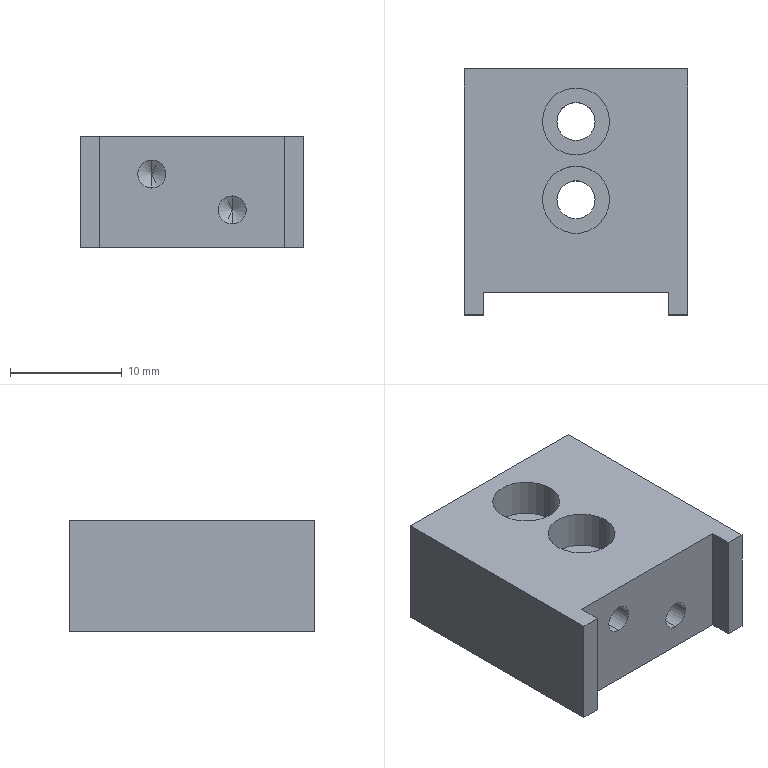Part | SolidWorks | features MBimport 1 | 1 solid | 35 faces | box 20 x 22 x 10 mm | volume 3468 mm3 | plane 16 | cylinder 15 | cone 4 | commonest cylinder face diameters 2.5 x4 3.4 x4 6 x4 3 x3
STEP:
#1=CARTESIAN_POINT('',(3.6,-5.,-0.35));
#2=VERTEX_POINT('',#1);
#3=CARTESIAN_POINT('',(3.6,-5.,-2.85));
#4=VERTEX_POINT('',#3);
#5=CARTESIAN_POINT('',(3.6,-5.,-1.6));
#6=DIRECTION('',(0.,-1.,0.));
#7=DIRECTION('',(0.,0.,-1.));
#8=AXIS2_PLACEMENT_3D('',#5,#6,#7);
#9=CIRCLE('',#8,1.25);
#10=EDGE_CURVE('',#2,#4,#9,.T.);
#11=ORIENTED_EDGE('',*,*,#10,.F.);
#12=CARTESIAN_POINT('',(3.6,-10.,-0.35));
#13=VERTEX_POINT('',#12);
#14=CARTESIAN_POINT('',(3.6,-10.,-0.35));
#15=DIRECTION('',(0.,-1.,0.));
#16=VECTOR('',#15,1000.);
#17=LINE('',#14,#16);
#18=EDGE_CURVE('',#2,#13,#17,.T.);
#19=ORIENTED_EDGE('',*,*,#18,.T.);
#20=CARTESIAN_POINT('',(3.6,-10.,-2.85));
#21=VERTEX_POINT('',#20);
#22=CARTESIAN_POINT('',(3.6,-10.,-1.6));
#23=DIRECTION('',(0.,-1.,0.));
#24=DIRECTION('',(0.,0.,-1.));
#25=AXIS2_PLACEMENT_3D('',#22,#23,#24);
#26=CIRCLE('',#25,1.25);
#27=EDGE_CURVE('',#13,#21,#26,.T.);
#28=ORIENTED_EDGE('',*,*,#27,.T.);
#29=CARTESIAN_POINT('',(3.6,-10.,-2.85));
#30=DIRECTION('',(0.,-1.,0.));
#31=VECTOR('',#30,1000.);
#32=LINE('',#29,#31);
#33=EDGE_CURVE('',#4,#21,#32,.T.);
#34=ORIENTED_EDGE('',*,*,#33,.F.);
#35=EDGE_LOOP('',(#11,#19,#28,#34));
#36=FACE_OUTER_BOUND('',#35,.T.);
#37=CARTESIAN_POINT('',(3.6,-10.,-1.6));
#38=DIRECTION('',(0.,-1.,0.));
#39=DIRECTION('',(0.,0.,-1.));
#40=AXIS2_PLACEMENT_3D('',#37,#38,#39);
#41=CYLINDRICAL_SURFACE('',#40,1.25);
#42=ADVANCED_FACE('',(#36),#41,.F.);
#43=CARTESIAN_POINT('',(3.6,-4.249,-1.6));
#44=VERTEX_POINT('',#43);
#45=CARTESIAN_POINT('',(3.6,-5.,-2.85));
#46=DIRECTION('',(0.,-0.515,-0.8572));
#47=VECTOR('',#46,1000.);
#48=LINE('',#45,#47);
#49=EDGE_CURVE('',#44,#4,#48,.T.);
#50=ORIENTED_EDGE('',*,*,#49,.F.);
#51=CARTESIAN_POINT('',(3.6,-5.,-0.35));
#52=DIRECTION('',(0.,-0.515,0.8572));
#53=VECTOR('',#52,1000.);
#54=LINE('',#51,#53);
#55=EDGE_CURVE('',#44,#2,#54,.T.);
#56=ORIENTED_EDGE('',*,*,#55,.T.);
#57=ORIENTED_EDGE('',*,*,#10,.T.);
#58=EDGE_LOOP('',(#50,#56,#57));
#59=FACE_OUTER_BOUND('',#58,.T.);
#60=CARTESIAN_POINT('',(3.6,-5.,-1.6));
#61=DIRECTION('',(0.,-1.,0.));
#62=DIRECTION('',(0.,0.,-1.));
#63=AXIS2_PLACEMENT_3D('',#60,#61,#62);
#64=CONICAL_SURFACE('',#63,1.25,1.03);
#65=ADVANCED_FACE('',(#59),#64,.F.);
#66=CARTESIAN_POINT('',(-3.6,-5.,2.85));
#67=VERTEX_POINT('',#66);
#68=CARTESIAN_POINT('',(-3.6,-5.,0.35));
#69=VERTEX_POINT('',#68);
#70=CARTESIAN_POINT('',(-3.6,-5.,1.6));
#71=DIRECTION('',(0.,-1.,0.));
#72=DIRECTION('',(0.,0.,-1.));
#73=AXIS2_PLACEMENT_3D('',#70,#71,#72);
#74=CIRCLE('',#73,1.25);
#75=EDGE_CURVE('',#67,#69,#74,.T.);
#76=ORIENTED_EDGE('',*,*,#75,.F.);
#77=CARTESIAN_POINT('',(-3.6,-10.,2.85));
#78=VERTEX_POINT('',#77);
#79=CARTESIAN_POINT('',(-3.6,-10.,2.85));
#80=DIRECTION('',(0.,-1.,0.));
#81=VECTOR('',#80,1000.);
#82=LINE('',#79,#81);
#83=EDGE_CURVE('',#67,#78,#82,.T.);
#84=ORIENTED_EDGE('',*,*,#83,.T.);
#85=CARTESIAN_POINT('',(-3.6,-10.,0.35));
#86=VERTEX_POINT('',#85);
#87=CARTESIAN_POINT('',(-3.6,-10.,1.6));
#88=DIRECTION('',(0.,-1.,0.));
#89=DIRECTION('',(0.,0.,-1.));
#90=AXIS2_PLACEMENT_3D('',#87,#88,#89);
#91=CIRCLE('',#90,1.25);
#92=EDGE_CURVE('',#78,#86,#91,.T.);
#93=ORIENTED_EDGE('',*,*,#92,.T.);
#94=CARTESIAN_POINT('',(-3.6,-10.,0.35));
#95=DIRECTION('',(0.,-1.,0.));
#96=VECTOR('',#95,1000.);
#97=LINE('',#94,#96);
#98=EDGE_CURVE('',#69,#86,#97,.T.);
#99=ORIENTED_EDGE('',*,*,#98,.F.);
#100=EDGE_LOOP('',(#76,#84,#93,#99));
#101=FACE_OUTER_BOUND('',#100,.T.);
#102=CARTESIAN_POINT('',(-3.6,-10.,1.6));
#103=DIRECTION('',(0.,-1.,0.));
#104=DIRECTION('',(0.,0.,-1.));
#105=AXIS2_PLACEMENT_3D('',#102,#103,#104);
#106=CYLINDRICAL_SURFACE('',#105,1.25);
#107=ADVANCED_FACE('',(#101),#106,.F.);
#108=CARTESIAN_POINT('',(-3.6,-4.249,1.6));
#109=VERTEX_POINT('',#108);
#110=CARTESIAN_POINT('',(-3.6,-5.,0.35));
#111=DIRECTION('',(0.,-0.515,-0.8572));
#112=VECTOR('',#111,1000.);
#113=LINE('',#110,#112);
#114=EDGE_CURVE('',#109,#69,#113,.T.);
#115=ORIENTED_EDGE('',*,*,#114,.F.);
#116=CARTESIAN_POINT('',(-3.6,-5.,2.85));
#117=DIRECTION('',(0.,-0.515,0.8572));
#118=VECTOR('',#117,1000.);
#119=LINE('',#116,#118);
#120=EDGE_CURVE('',#109,#67,#119,.T.);
#121=ORIENTED_EDGE('',*,*,#120,.T.);
#122=ORIENTED_EDGE('',*,*,#75,.T.);
#123=EDGE_LOOP('',(#115,#121,#122));
#124=FACE_OUTER_BOUND('',#123,.T.);
#125=CARTESIAN_POINT('',(-3.6,-5.,1.6));
#126=DIRECTION('',(0.,-1.,0.));
#127=DIRECTION('',(0.,0.,-1.));
#128=AXIS2_PLACEMENT_3D('',#125,#126,#127);
#129=CONICAL_SURFACE('',#128,1.25,1.03);
#130=ADVANCED_FACE('',(#124),#129,.F.);
#131=CARTESIAN_POINT('',(-4.,-4.2,-3.));
#132=VERTEX_POINT('',#131);
#133=CARTESIAN_POINT('',(-5.5,-5.7,-3.));
#134=VERTEX_POINT('',#133);
#135=CARTESIAN_POINT('',(-4.,-5.7,-3.));
#136=DIRECTION('',(0.,0.,1.));
#137=DIRECTION('',(-1.,0.,0.));
#138=AXIS2_PLACEMENT_3D('',#135,#136,#137);
#139=CIRCLE('',#138,1.5);
#140=EDGE_CURVE('',#132,#134,#139,.T.);
#141=ORIENTED_EDGE('',*,*,#140,.T.);
#142=CARTESIAN_POINT('',(-5.5,-5.7,-5.));
#143=VERTEX_POINT('',#142);
#144=CARTESIAN_POINT('',(-5.5,-5.7,1.243));
#145=DIRECTION('',(0.,0.,-1.));
#146=VECTOR('',#145,1000.);
#147=LINE('',#144,#146);
#148=EDGE_CURVE('',#134,#143,#147,.T.);
#149=ORIENTED_EDGE('',*,*,#148,.T.);
#150=CARTESIAN_POINT('',(-4.,-4.2,-5.));
#151=VERTEX_POINT('',#150);
#152=CARTESIAN_POINT('',(-4.,-5.7,-5.));
#153=DIRECTION('',(0.,0.,-1.));
#154=DIRECTION('',(-1.,0.,0.));
#155=AXIS2_PLACEMENT_3D('',#152,#153,#154);
#156=CIRCLE('',#155,1.5);
#157=EDGE_CURVE('',#143,#151,#156,.T.);
#158=ORIENTED_EDGE('',*,*,#157,.T.);
#159=CARTESIAN_POINT('',(-4.,-4.2,1.243));
#160=DIRECTION('',(0.,0.,-1.));
#161=VECTOR('',#160,1000.);
#162=LINE('',#159,#161);
#163=EDGE_CURVE('',#132,#151,#162,.T.);
#164=ORIENTED_EDGE('',*,*,#163,.F.);
#165=EDGE_LOOP('',(#141,#149,#158,#164));
#166=FACE_OUTER_BOUND('',#165,.T.);
#167=CARTESIAN_POINT('',(-4.,-5.7,1.243));
#168=DIRECTION('',(0.,0.,-1.));
#169=DIRECTION('',(-1.,0.,0.));
#170=AXIS2_PLACEMENT_3D('',#167,#168,#169);
#171=CYLINDRICAL_SURFACE('',#170,1.5);
#172=ADVANCED_FACE('',(#166),#171,.F.);
#173=CARTESIAN_POINT('',(-3.,5.3,1.6));
#174=VERTEX_POINT('',#173);
#175=CARTESIAN_POINT('',(3.,5.3,1.6));
#176=VERTEX_POINT('',#175);
#177=CARTESIAN_POINT('',(0.,5.3,1.6));
#178=DIRECTION('',(0.,0.,1.));
#179=DIRECTION('',(1.,0.,0.));
#180=AXIS2_PLACEMENT_3D('',#177,#178,#179);
#181=CIRCLE('',#180,3.);
#182=EDGE_CURVE('',#174,#176,#181,.T.);
#183=ORIENTED_EDGE('',*,*,#182,.F.);
#184=CARTESIAN_POINT('',(-3.,5.3,5.));
#185=VERTEX_POINT('',#184);
#186=CARTESIAN_POINT('',(-3.,5.3,5.));
#187=DIRECTION('',(0.,0.,1.));
#188=VECTOR('',#187,1000.);
#189=LINE('',#186,#188);
#190=EDGE_CURVE('',#174,#185,#189,.T.);
#191=ORIENTED_EDGE('',*,*,#190,.T.);
#192=CARTESIAN_POINT('',(3.,5.3,5.));
#193=VERTEX_POINT('',#192);
#194=CARTESIAN_POINT('',(0.,5.3,5.));
#195=DIRECTION('',(0.,0.,1.));
#196=DIRECTION('',(1.,0.,0.));
#197=AXIS2_PLACEMENT_3D('',#194,#195,#196);
#198=CIRCLE('',#197,3.);
#199=EDGE_CURVE('',#185,#193,#198,.T.);
#200=ORIENTED_EDGE('',*,*,#199,.T.);
#201=CARTESIAN_POINT('',(3.,5.3,5.));
#202=DIRECTION('',(0.,0.,1.));
#203=VECTOR('',#202,1000.);
#204=LINE('',#201,#203);
#205=EDGE_CURVE('',#176,#193,#204,.T.);
#206=ORIENTED_EDGE('',*,*,#205,.F.);
#207=EDGE_LOOP('',(#183,#191,#200,#206));
#208=FACE_OUTER_BOUND('',#207,.T.);
#209=CARTESIAN_POINT('',(0.,5.3,5.));
#210=DIRECTION('',(0.,0.,1.));
#211=DIRECTION('',(1.,0.,0.));
#212=AXIS2_PLACEMENT_3D('',#209,#210,#211);
#213=CYLINDRICAL_SURFACE('',#212,3.);
#214=ADVANCED_FACE('',(#208),#213,.F.);
#215=CARTESIAN_POINT('',(1.7,5.3,-3.));
#216=VERTEX_POINT('',#215);
#217=CARTESIAN_POINT('',(-1.7,5.3,-3.));
#218=VERTEX_POINT('',#217);
#219=CARTESIAN_POINT('',(0.,5.3,-3.));
#220=DIRECTION('',(0.,0.,-1.));
#221=DIRECTION('',(-1.,0.,0.));
#222=AXIS2_PLACEMENT_3D('',#219,#220,#221);
#223=CIRCLE('',#222,1.7);
#224=EDGE_CURVE('',#216,#218,#223,.T.);
#225=ORIENTED_EDGE('',*,*,#224,.T.);
#226=CARTESIAN_POINT('',(-1.7,5.3,1.6));
#227=VERTEX_POINT('',#226);
#228=CARTESIAN_POINT('',(-1.7,5.3,5.));
#229=DIRECTION('',(0.,0.,1.));
#230=VECTOR('',#229,1000.);
#231=LINE('',#228,#230);
#232=EDGE_CURVE('',#218,#227,#231,.T.);
#233=ORIENTED_EDGE('',*,*,#232,.T.);
#234=CARTESIAN_POINT('',(1.7,5.3,1.6));
#235=VERTEX_POINT('',#234);
#236=CARTESIAN_POINT('',(0.,5.3,1.6));
#237=DIRECTION('',(0.,0.,1.));
#238=DIRECTION('',(1.,0.,0.));
#239=AXIS2_PLACEMENT_3D('',#236,#237,#238);
#240=CIRCLE('',#239,1.7);
#241=EDGE_CURVE('',#227,#235,#240,.T.);
#242=ORIENTED_EDGE('',*,*,#241,.T.);
#243=CARTESIAN_POINT('',(1.7,5.3,5.));
#244=DIRECTION('',(0.,0.,1.));
#245=VECTOR('',#244,1000.);
#246=LINE('',#243,#245);
#247=EDGE_CURVE('',#216,#235,#246,.T.);
#248=ORIENTED_EDGE('',*,*,#247,.F.);
#249=EDGE_LOOP('',(#225,#233,#242,#248));
#250=FACE_OUTER_BOUND('',#249,.T.);
#251=CARTESIAN_POINT('',(0.,5.3,5.));
#252=DIRECTION('',(0.,0.,1.));
#253=DIRECTION('',(1.,0.,0.));
#254=AXIS2_PLACEMENT_3D('',#251,#252,#253);
#255=CYLINDRICAL_SURFACE('',#254,1.7);
#256=ADVANCED_FACE('',(#250),#255,.F.);
#257=CARTESIAN_POINT('',(-3.,-1.7,1.6));
#258=VERTEX_POINT('',#257);
#259=CARTESIAN_POINT('',(3.,-1.7,1.6));
#260=VERTEX_POINT('',#259);
#261=CARTESIAN_POINT('',(0.,-1.7,1.6));
#262=DIRECTION('',(0.,0.,1.));
#263=DIRECTION('',(1.,0.,0.));
#264=AXIS2_PLACEMENT_3D('',#261,#262,#263);
#265=CIRCLE('',#264,3.);
#266=EDGE_CURVE('',#258,#260,#265,.T.);
#267=ORIENTED_EDGE('',*,*,#266,.F.);
#268=CARTESIAN_POINT('',(-3.,-1.7,5.));
#269=VERTEX_POINT('',#268);
#270=CARTESIAN_POINT('',(-3.,-1.7,5.));
#271=DIRECTION('',(0.,0.,1.));
#272=VECTOR('',#271,1000.);
#273=LINE('',#270,#272);
#274=EDGE_CURVE('',#258,#269,#273,.T.);
#275=ORIENTED_EDGE('',*,*,#274,.T.);
#276=CARTESIAN_POINT('',(3.,-1.7,5.));
#277=VERTEX_POINT('',#276);
#278=CARTESIAN_POINT('',(0.,-1.7,5.));
#279=DIRECTION('',(0.,0.,1.));
#280=DIRECTION('',(1.,0.,0.));
#281=AXIS2_PLACEMENT_3D('',#278,#279,#280);
#282=CIRCLE('',#281,3.);
#283=EDGE_CURVE('',#269,#277,#282,.T.);
#284=ORIENTED_EDGE('',*,*,#283,.T.);
#285=CARTESIAN_POINT('',(3.,-1.7,5.));
#286=DIRECTION('',(0.,0.,1.));
#287=VECTOR('',#286,1000.);
#288=LINE('',#285,#287);
#289=EDGE_CURVE('',#260,#277,#288,.T.);
#290=ORIENTED_EDGE('',*,*,#289,.F.);
#291=EDGE_LOOP('',(#267,#275,#284,#290));
#292=FACE_OUTER_BOUND('',#291,.T.);
#293=CARTESIAN_POINT('',(0.,-1.7,5.));
#294=DIRECTION('',(0.,0.,1.));
#295=DIRECTION('',(1.,0.,0.));
#296=AXIS2_PLACEMENT_3D('',#293,#294,#295);
#297=CYLINDRICAL_SURFACE('',#296,3.);
#298=ADVANCED_FACE('',(#292),#297,.F.);
#299=CARTESIAN_POINT('',(1.7,-1.7,-3.));
#300=VERTEX_POINT('',#299);
#301=CARTESIAN_POINT('',(-1.7,-1.7,-3.));
#302=VERTEX_POINT('',#301);
#303=CARTESIAN_POINT('',(0.,-1.7,-3.));
#304=DIRECTION('',(0.,0.,-1.));
#305=DIRECTION('',(-1.,0.,0.));
#306=AXIS2_PLACEMENT_3D('',#303,#304,#305);
#307=CIRCLE('',#306,1.7);
#308=EDGE_CURVE('',#300,#302,#307,.T.);
#309=ORIENTED_EDGE('',*,*,#308,.T.);
#310=CARTESIAN_POINT('',(-1.7,-1.7,1.6));
#311=VERTEX_POINT('',#310);
#312=CARTESIAN_POINT('',(-1.7,-1.7,5.));
#313=DIRECTION('',(0.,0.,1.));
#314=VECTOR('',#313,1000.);
#315=LINE('',#312,#314);
#316=EDGE_CURVE('',#302,#311,#315,.T.);
#317=ORIENTED_EDGE('',*,*,#316,.T.);
#318=CARTESIAN_POINT('',(1.7,-1.7,1.6));
#319=VERTEX_POINT('',#318);
#320=CARTESIAN_POINT('',(0.,-1.7,1.6));
#321=DIRECTION('',(0.,0.,1.));
#322=DIRECTION('',(1.,0.,0.));
#323=AXIS2_PLACEMENT_3D('',#320,#321,#322);
#324=CIRCLE('',#323,1.7);
#325=EDGE_CURVE('',#311,#319,#324,.T.);
#326=ORIENTED_EDGE('',*,*,#325,.T.);
#327=CARTESIAN_POINT('',(1.7,-1.7,5.));
#328=DIRECTION('',(0.,0.,1.));
#329=VECTOR('',#328,1000.);
#330=LINE('',#327,#329);
#331=EDGE_CURVE('',#300,#319,#330,.T.);
#332=ORIENTED_EDGE('',*,*,#331,.F.);
#333=EDGE_LOOP('',(#309,#317,#326,#332));
#334=FACE_OUTER_BOUND('',#333,.T.);
#335=CARTESIAN_POINT('',(0.,-1.7,5.));
#336=DIRECTION('',(0.,0.,1.));
#337=DIRECTION('',(1.,0.,0.));
#338=AXIS2_PLACEMENT_3D('',#335,#336,#337);
#339=CYLINDRICAL_SURFACE('',#338,1.7);
#340=ADVANCED_FACE('',(#334),#339,.F.);
#341=CARTESIAN_POINT('',(8.3,-10.,5.));
#342=VERTEX_POINT('',#341);
#343=CARTESIAN_POINT('',(8.3,-10.,-5.));
#344=VERTEX_POINT('',#343);
#345=CARTESIAN_POINT('',(8.3,-10.,5.));
#346=DIRECTION('',(0.,0.,-1.));
#347=VECTOR('',#346,1000.);
#348=LINE('',#345,#347);
#349=EDGE_CURVE('',#342,#344,#348,.T.);
#350=ORIENTED_EDGE('',*,*,#349,.F.);
#351=CARTESIAN_POINT('',(-8.3,-10.,5.));
#352=VERTEX_POINT('',#351);
#353=CARTESIAN_POINT('',(-10.,-10.,5.));
#354=DIRECTION('',(1.,0.,0.));
#355=VECTOR('',#354,1000.);
#356=LINE('',#353,#355);
#357=EDGE_CURVE('',#352,#342,#356,.T.);
#358=ORIENTED_EDGE('',*,*,#357,.F.);
#359=CARTESIAN_POINT('',(-8.3,-10.,-5.));
#360=VERTEX_POINT('',#359);
#361=CARTESIAN_POINT('',(-8.3,-10.,5.));
#362=DIRECTION('',(0.,0.,1.));
#363=VECTOR('',#362,1000.);
#364=LINE('',#361,#363);
#365=EDGE_CURVE('',#360,#352,#364,.T.);
#366=ORIENTED_EDGE('',*,*,#365,.F.);
#367=CARTESIAN_POINT('',(-10.,-10.,-5.));
#368=DIRECTION('',(1.,0.,0.));
#369=VECTOR('',#368,1000.);
#370=LINE('',#367,#369);
#371=EDGE_CURVE('',#360,#344,#370,.T.);
#372=ORIENTED_EDGE('',*,*,#371,.T.);
#373=EDGE_LOOP('',(#350,#358,#366,#372));
#374=FACE_OUTER_BOUND('',#373,.T.);
#375=CARTESIAN_POINT('',(3.6,-10.,-1.6));
#376=DIRECTION('',(0.,-1.,0.));
#377=DIRECTION('',(0.,0.,-1.));
#378=AXIS2_PLACEMENT_3D('',#375,#376,#377);
#379=CIRCLE('',#378,1.25);
#380=EDGE_CURVE('',#21,#13,#379,.T.);
#381=ORIENTED_EDGE('',*,*,#380,.F.);
#382=ORIENTED_EDGE('',*,*,#27,.F.);
#383=EDGE_LOOP('',(#381,#382));
#384=FACE_BOUND('',#383,.T.);
#385=CARTESIAN_POINT('',(-3.6,-10.,1.6));
#386=DIRECTION('',(0.,-1.,0.));
#387=DIRECTION('',(0.,0.,-1.));
#388=AXIS2_PLACEMENT_3D('',#385,#386,#387);
#389=CIRCLE('',#388,1.25);
#390=EDGE_CURVE('',#86,#78,#389,.T.);
#391=ORIENTED_EDGE('',*,*,#390,.F.);
#392=ORIENTED_EDGE('',*,*,#92,.F.);
#393=EDGE_LOOP('',(#391,#392));
#394=FACE_BOUND('',#393,.T.);
#395=CARTESIAN_POINT('',(-10.,-10.,5.));
#396=DIRECTION('',(0.,1.,0.));
#397=DIRECTION('',(1.,0.,0.));
#398=AXIS2_PLACEMENT_3D('',#395,#396,#397);
#399=PLANE('',#398);
#400=ADVANCED_FACE('',(#374,#384,#394),#399,.F.);
#401=CARTESIAN_POINT('',(10.,-12.,-5.));
#402=VERTEX_POINT('',#401);
#403=CARTESIAN_POINT('',(10.,10.,-5.));
#404=VERTEX_POINT('',#403);
#405=CARTESIAN_POINT('',(10.,10.,-5.));
#406=DIRECTION('',(0.,1.,0.));
#407=VECTOR('',#406,1000.);
#408=LINE('',#405,#407);
#409=EDGE_CURVE('',#402,#404,#408,.T.);
#410=ORIENTED_EDGE('',*,*,#409,.T.);
#411=CARTESIAN_POINT('',(10.,10.,5.));
#412=VERTEX_POINT('',#411);
#413=CARTESIAN_POINT('',(10.,10.,5.));
#414=DIRECTION('',(0.,0.,-1.));
#415=VECTOR('',#414,1000.);
#416=LINE('',#413,#415);
#417=EDGE_CURVE('',#412,#404,#416,.T.);
#418=ORIENTED_EDGE('',*,*,#417,.F.);
#419=CARTESIAN_POINT('',(10.,-12.,5.));
#420=VERTEX_POINT('',#419);
#421=CARTESIAN_POINT('',(10.,10.,5.));
#422=DIRECTION('',(0.,1.,0.));
#423=VECTOR('',#422,1000.);
#424=LINE('',#421,#423);
#425=EDGE_CURVE('',#420,#412,#424,.T.);
#426=ORIENTED_EDGE('',*,*,#425,.F.);
#427=CARTESIAN_POINT('',(10.,-12.,5.));
#428=DIRECTION('',(0.,0.,1.));
#429=VECTOR('',#428,1000.);
#430=LINE('',#427,#429);
#431=EDGE_CURVE('',#402,#420,#430,.T.);
#432=ORIENTED_EDGE('',*,*,#431,.F.);
#433=EDGE_LOOP('',(#410,#418,#426,#432));
#434=FACE_OUTER_BOUND('',#433,.T.);
#435=CARTESIAN_POINT('',(10.,10.,5.));
#436=DIRECTION('',(-1.,0.,0.));
#437=DIRECTION('',(0.,1.,0.));
#438=AXIS2_PLACEMENT_3D('',#435,#436,#437);
#439=PLANE('',#438);
#440=ADVANCED_FACE('',(#434),#439,.F.);
#441=CARTESIAN_POINT('',(-4.,10.,-3.));
#442=VERTEX_POINT('',#441);
#443=CARTESIAN_POINT('',(4.,10.,-3.));
#444=VERTEX_POINT('',#443);
#445=CARTESIAN_POINT('',(-10.,10.,-3.));
#446=DIRECTION('',(1.,0.,0.));
#447=VECTOR('',#446,1000.);
#448=LINE('',#445,#447);
#449=EDGE_CURVE('',#442,#444,#448,.T.);
#450=ORIENTED_EDGE('',*,*,#449,.F.);
#451=CARTESIAN_POINT('',(-4.,10.,-5.));
#452=VERTEX_POINT('',#451);
#453=CARTESIAN_POINT('',(-4.,10.,5.));
#454=DIRECTION('',(0.,0.,-1.));
#455=VECTOR('',#454,1000.);
#456=LINE('',#453,#455);
#457=EDGE_CURVE('',#442,#452,#456,.T.);
#458=ORIENTED_EDGE('',*,*,#457,.T.);
#459=CARTESIAN_POINT('',(-10.,10.,-5.));
#460=VERTEX_POINT('',#459);
#461=CARTESIAN_POINT('',(-10.,10.,-5.));
#462=DIRECTION('',(-1.,0.,0.));
#463=VECTOR('',#462,1000.);
#464=LINE('',#461,#463);
#465=EDGE_CURVE('',#452,#460,#464,.T.);
#466=ORIENTED_EDGE('',*,*,#465,.T.);
#467=CARTESIAN_POINT('',(-10.,10.,5.));
#468=VERTEX_POINT('',#467);
#469=CARTESIAN_POINT('',(-10.,10.,5.));
#470=DIRECTION('',(0.,0.,-1.));
#471=VECTOR('',#470,1000.);
#472=LINE('',#469,#471);
#473=EDGE_CURVE('',#468,#460,#472,.T.);
#474=ORIENTED_EDGE('',*,*,#473,.F.);
#475=CARTESIAN_POINT('',(-10.,10.,5.));
#476=DIRECTION('',(-1.,0.,0.));
#477=VECTOR('',#476,1000.);
#478=LINE('',#475,#477);
#479=EDGE_CURVE('',#412,#468,#478,.T.);
#480=ORIENTED_EDGE('',*,*,#479,.F.);
#481=ORIENTED_EDGE('',*,*,#417,.T.);
#482=CARTESIAN_POINT('',(4.,10.,-5.));
#483=VERTEX_POINT('',#482);
#484=CARTESIAN_POINT('',(-10.,10.,-5.));
#485=DIRECTION('',(-1.,0.,0.));
#486=VECTOR('',#485,1000.);
#487=LINE('',#484,#486);
#488=EDGE_CURVE('',#404,#483,#487,.T.);
#489=ORIENTED_EDGE('',*,*,#488,.T.);
#490=CARTESIAN_POINT('',(4.,10.,5.));
#491=DIRECTION('',(0.,0.,1.));
#492=VECTOR('',#491,1000.);
#493=LINE('',#490,#492);
#494=EDGE_CURVE('',#483,#444,#493,.T.);
#495=ORIENTED_EDGE('',*,*,#494,.T.);
#496=EDGE_LOOP('',(#450,#458,#466,#474,#480,#481,#489,#495));
#497=FACE_OUTER_BOUND('',#496,.T.);
#498=CARTESIAN_POINT('',(-10.,10.,5.));
#499=DIRECTION('',(0.,-1.,0.));
#500=DIRECTION('',(0.,0.,-1.));
#501=AXIS2_PLACEMENT_3D('',#498,#499,#500);
#502=PLANE('',#501);
#503=ADVANCED_FACE('',(#497),#502,.F.);
#504=CARTESIAN_POINT('',(-10.,-12.,-5.));
#505=VERTEX_POINT('',#504);
#506=CARTESIAN_POINT('',(-10.,10.,-5.));
#507=DIRECTION('',(0.,-1.,0.));
#508=VECTOR('',#507,1000.);
#509=LINE('',#506,#508);
#510=EDGE_CURVE('',#460,#505,#509,.T.);
#511=ORIENTED_EDGE('',*,*,#510,.T.);
#512=CARTESIAN_POINT('',(-10.,-12.,5.));
#513=VERTEX_POINT('',#512);
#514=CARTESIAN_POINT('',(-10.,-12.,5.));
#515=DIRECTION('',(0.,0.,-1.));
#516=VECTOR('',#515,1000.);
#517=LINE('',#514,#516);
#518=EDGE_CURVE('',#513,#505,#517,.T.);
#519=ORIENTED_EDGE('',*,*,#518,.F.);
#520=CARTESIAN_POINT('',(-10.,10.,5.));
#521=DIRECTION('',(0.,-1.,0.));
#522=VECTOR('',#521,1000.);
#523=LINE('',#520,#522);
#524=EDGE_CURVE('',#468,#513,#523,.T.);
#525=ORIENTED_EDGE('',*,*,#524,.F.);
#526=ORIENTED_EDGE('',*,*,#473,.T.);
#527=EDGE_LOOP('',(#511,#519,#525,#526));
#528=FACE_OUTER_BOUND('',#527,.T.);
#529=CARTESIAN_POINT('',(-10.,10.,5.));
#530=DIRECTION('',(1.,0.,0.));
#531=DIRECTION('',(0.,1.,0.));
#532=AXIS2_PLACEMENT_3D('',#529,#530,#531);
#533=PLANE('',#532);
#534=ADVANCED_FACE('',(#528),#533,.F.);
#535=ORIENTED_EDGE('',*,*,#425,.T.);
#536=ORIENTED_EDGE('',*,*,#479,.T.);
#537=ORIENTED_EDGE('',*,*,#524,.T.);
#538=CARTESIAN_POINT('',(-8.3,-12.,5.));
#539=VERTEX_POINT('',#538);
#540=CARTESIAN_POINT('',(-10.,-12.,5.));
#541=DIRECTION('',(-1.,0.,0.));
#542=VECTOR('',#541,1000.);
#543=LINE('',#540,#542);
#544=EDGE_CURVE('',#539,#513,#543,.T.);
#545=ORIENTED_EDGE('',*,*,#544,.F.);
#546=CARTESIAN_POINT('',(-8.3,-12.,5.));
#547=DIRECTION('',(0.,1.,0.));
#548=VECTOR('',#547,1000.);
#549=LINE('',#546,#548);
#550=EDGE_CURVE('',#539,#352,#549,.T.);
#551=ORIENTED_EDGE('',*,*,#550,.T.);
#552=ORIENTED_EDGE('',*,*,#357,.T.);
#553=CARTESIAN_POINT('',(8.3,-12.,5.));
#554=VERTEX_POINT('',#553);
#555=CARTESIAN_POINT('',(8.3,-12.,5.));
#556=DIRECTION('',(0.,1.,0.));
#557=VECTOR('',#556,1000.);
#558=LINE('',#555,#557);
#559=EDGE_CURVE('',#554,#342,#558,.T.);
#560=ORIENTED_EDGE('',*,*,#559,.F.);
#561=CARTESIAN_POINT('',(10.,-12.,5.));
#562=DIRECTION('',(-1.,0.,0.));
#563=VECTOR('',#562,1000.);
#564=LINE('',#561,#563);
#565=EDGE_CURVE('',#420,#554,#564,.T.);
#566=ORIENTED_EDGE('',*,*,#565,.F.);
#567=EDGE_LOOP('',(#535,#536,#537,#545,#551,#552,#560,#566));
#568=FACE_OUTER_BOUND('',#567,.T.);
#569=CARTESIAN_POINT('',(0.,5.3,5.));
#570=DIRECTION('',(0.,0.,1.));
#571=DIRECTION('',(1.,0.,0.));
#572=AXIS2_PLACEMENT_3D('',#569,#570,#571);
#573=CIRCLE('',#572,3.);
#574=EDGE_CURVE('',#193,#185,#573,.T.);
#575=ORIENTED_EDGE('',*,*,#574,.F.);
#576=ORIENTED_EDGE('',*,*,#199,.F.);
#577=EDGE_LOOP('',(#575,#576));
#578=FACE_BOUND('',#577,.T.);
#579=CARTESIAN_POINT('',(0.,-1.7,5.));
#580=DIRECTION('',(0.,0.,1.));
#581=DIRECTION('',(1.,0.,0.));
#582=AXIS2_PLACEMENT_3D('',#579,#580,#581);
#583=CIRCLE('',#582,3.);
#584=EDGE_CURVE('',#277,#269,#583,.T.);
#585=ORIENTED_EDGE('',*,*,#584,.F.);
#586=ORIENTED_EDGE('',*,*,#283,.F.);
#587=EDGE_LOOP('',(#585,#586));
#588=FACE_BOUND('',#587,.T.);
#589=CARTESIAN_POINT('',(0.,0.,5.));
#590=DIRECTION('',(0.,0.,1.));
#591=DIRECTION('',(1.,0.,0.));
#592=AXIS2_PLACEMENT_3D('',#589,#590,#591);
#593=PLANE('',#592);
#594=ADVANCED_FACE('',(#568,#578,#588),#593,.T.);
#595=CARTESIAN_POINT('',(2.5,-5.7,-5.));
#596=VERTEX_POINT('',#595);
#597=CARTESIAN_POINT('',(-2.5,-5.7,-5.));
#598=VERTEX_POINT('',#597);
#599=CARTESIAN_POINT('',(4.,-5.7,-5.));
#600=DIRECTION('',(-1.,0.,0.));
#601=VECTOR('',#600,1000.);
#602=LINE('',#599,#601);
#603=EDGE_CURVE('',#596,#598,#602,.T.);
#604=ORIENTED_EDGE('',*,*,#603,.F.);
#605=CARTESIAN_POINT('',(4.,-4.2,-5.));
#606=VERTEX_POINT('',#605);
#607=CARTESIAN_POINT('',(4.,-5.7,-5.));
#608=DIRECTION('',(0.,0.,-1.));
#609=DIRECTION('',(-1.,0.,0.));
#610=AXIS2_PLACEMENT_3D('',#607,#608,#609);
#611=CIRCLE('',#610,1.5);
#612=EDGE_CURVE('',#606,#596,#611,.T.);
#613=ORIENTED_EDGE('',*,*,#612,.F.);
#614=CARTESIAN_POINT('',(4.,0.,-5.));
#615=DIRECTION('',(0.,1.,0.));
#616=VECTOR('',#615,1000.);
#617=LINE('',#614,#616);
#618=EDGE_CURVE('',#606,#483,#617,.T.);
#619=ORIENTED_EDGE('',*,*,#618,.T.);
#620=ORIENTED_EDGE('',*,*,#488,.F.);
#621=ORIENTED_EDGE('',*,*,#409,.F.);
#622=CARTESIAN_POINT('',(8.3,-12.,-5.));
#623=VERTEX_POINT('',#622);
#624=CARTESIAN_POINT('',(10.,-12.,-5.));
#625=DIRECTION('',(1.,0.,0.));
#626=VECTOR('',#625,1000.);
#627=LINE('',#624,#626);
#628=EDGE_CURVE('',#623,#402,#627,.T.);
#629=ORIENTED_EDGE('',*,*,#628,.F.);
#630=CARTESIAN_POINT('',(8.3,-12.,-5.));
#631=DIRECTION('',(0.,1.,0.));
#632=VECTOR('',#631,1000.);
#633=LINE('',#630,#632);
#634=EDGE_CURVE('',#623,#344,#633,.T.);
#635=ORIENTED_EDGE('',*,*,#634,.T.);
#636=ORIENTED_EDGE('',*,*,#371,.F.);
#637=CARTESIAN_POINT('',(-8.3,-12.,-5.));
#638=VERTEX_POINT('',#637);
#639=CARTESIAN_POINT('',(-8.3,-12.,-5.));
#640=DIRECTION('',(0.,1.,0.));
#641=VECTOR('',#640,1000.);
#642=LINE('',#639,#641);
#643=EDGE_CURVE('',#638,#360,#642,.T.);
#644=ORIENTED_EDGE('',*,*,#643,.F.);
#645=CARTESIAN_POINT('',(-10.,-12.,-5.));
#646=DIRECTION('',(1.,0.,0.));
#647=VECTOR('',#646,1000.);
#648=LINE('',#645,#647);
#649=EDGE_CURVE('',#505,#638,#648,.T.);
#650=ORIENTED_EDGE('',*,*,#649,.F.);
#651=ORIENTED_EDGE('',*,*,#510,.F.);
#652=ORIENTED_EDGE('',*,*,#465,.F.);
#653=CARTESIAN_POINT('',(-4.,25.7,-5.));
#654=DIRECTION('',(0.,1.,0.));
#655=VECTOR('',#654,1000.);
#656=LINE('',#653,#655);
#657=EDGE_CURVE('',#151,#452,#656,.T.);
#658=ORIENTED_EDGE('',*,*,#657,.F.);
#659=ORIENTED_EDGE('',*,*,#157,.F.);
#660=CARTESIAN_POINT('',(-4.,-5.7,-5.));
#661=DIRECTION('',(0.,0.,-1.));
#662=DIRECTION('',(-1.,0.,0.));
#663=AXIS2_PLACEMENT_3D('',#660,#661,#662);
#664=CIRCLE('',#663,1.5);
#665=EDGE_CURVE('',#598,#143,#664,.T.);
#666=ORIENTED_EDGE('',*,*,#665,.F.);
#667=EDGE_LOOP('',(#604,#613,#619,#620,#621,#629,#635,#636,#644,#650,#651,#652,#658,#659,#666));
#668=FACE_OUTER_BOUND('',#667,.T.);
#669=CARTESIAN_POINT('',(0.,0.,-5.));
#670=DIRECTION('',(0.,0.,1.));
#671=DIRECTION('',(1.,0.,0.));
#672=AXIS2_PLACEMENT_3D('',#669,#670,#671);
#673=PLANE('',#672);
#674=ADVANCED_FACE('',(#668),#673,.F.);
#675=CARTESIAN_POINT('',(4.,-4.2,-3.));
#676=VERTEX_POINT('',#675);
#677=CARTESIAN_POINT('',(4.,25.7,-3.));
#678=DIRECTION('',(0.,-1.,0.));
#679=VECTOR('',#678,1000.);
#680=LINE('',#677,#679);
#681=EDGE_CURVE('',#444,#676,#680,.T.);
#682=ORIENTED_EDGE('',*,*,#681,.T.);
#683=CARTESIAN_POINT('',(2.5,-5.7,-3.));
#684=VERTEX_POINT('',#683);
#685=CARTESIAN_POINT('',(4.,-5.7,-3.));
#686=DIRECTION('',(0.,0.,1.));
#687=DIRECTION('',(-1.,0.,0.));
#688=AXIS2_PLACEMENT_3D('',#685,#686,#687);
#689=CIRCLE('',#688,1.5);
#690=EDGE_CURVE('',#684,#676,#689,.T.);
#691=ORIENTED_EDGE('',*,*,#690,.F.);
#692=CARTESIAN_POINT('',(-2.5,-5.7,-3.));
#693=VERTEX_POINT('',#692);
#694=CARTESIAN_POINT('',(4.,-5.7,-3.));
#695=DIRECTION('',(-1.,0.,0.));
#696=VECTOR('',#695,1000.);
#697=LINE('',#694,#696);
#698=EDGE_CURVE('',#684,#693,#697,.T.);
#699=ORIENTED_EDGE('',*,*,#698,.T.);
#700=CARTESIAN_POINT('',(-4.,-5.7,-3.));
#701=DIRECTION('',(0.,0.,1.));
#702=DIRECTION('',(-1.,0.,0.));
#703=AXIS2_PLACEMENT_3D('',#700,#701,#702);
#704=CIRCLE('',#703,1.5);
#705=EDGE_CURVE('',#134,#693,#704,.T.);
#706=ORIENTED_EDGE('',*,*,#705,.F.);
#707=ORIENTED_EDGE('',*,*,#140,.F.);
#708=CARTESIAN_POINT('',(-4.,25.7,-3.));
#709=DIRECTION('',(0.,1.,0.));
#710=VECTOR('',#709,1000.);
#711=LINE('',#708,#710);
#712=EDGE_CURVE('',#132,#442,#711,.T.);
#713=ORIENTED_EDGE('',*,*,#712,.T.);
#714=ORIENTED_EDGE('',*,*,#449,.T.);
#715=EDGE_LOOP('',(#682,#691,#699,#706,#707,#713,#714));
#716=FACE_OUTER_BOUND('',#715,.T.);
#717=ORIENTED_EDGE('',*,*,#224,.F.);
#718=CARTESIAN_POINT('',(0.,5.3,-3.));
#719=DIRECTION('',(0.,0.,-1.));
#720=DIRECTION('',(-1.,0.,0.));
#721=AXIS2_PLACEMENT_3D('',#718,#719,#720);
#722=CIRCLE('',#721,1.7);
#723=EDGE_CURVE('',#218,#216,#722,.T.);
#724=ORIENTED_EDGE('',*,*,#723,.F.);
#725=EDGE_LOOP('',(#717,#724));
#726=FACE_BOUND('',#725,.T.);
#727=ORIENTED_EDGE('',*,*,#308,.F.);
#728=CARTESIAN_POINT('',(0.,-1.7,-3.));
#729=DIRECTION('',(0.,0.,-1.));
#730=DIRECTION('',(-1.,0.,0.));
#731=AXIS2_PLACEMENT_3D('',#728,#729,#730);
#732=CIRCLE('',#731,1.7);
#733=EDGE_CURVE('',#302,#300,#732,.T.);
#734=ORIENTED_EDGE('',*,*,#733,.F.);
#735=EDGE_LOOP('',(#727,#734));
#736=FACE_BOUND('',#735,.T.);
#737=CARTESIAN_POINT('',(0.,0.,-3.));
#738=DIRECTION('',(0.,0.,-1.));
#739=DIRECTION('',(0.,-1.,0.));
#740=AXIS2_PLACEMENT_3D('',#737,#738,#739);
#741=PLANE('',#740);
#742=ADVANCED_FACE('',(#716,#726,#736),#741,.T.);
#743=ORIENTED_EDGE('',*,*,#712,.F.);
#744=ORIENTED_EDGE('',*,*,#163,.T.);
#745=ORIENTED_EDGE('',*,*,#657,.T.);
#746=ORIENTED_EDGE('',*,*,#457,.F.);
#747=EDGE_LOOP('',(#743,#744,#745,#746));
#748=FACE_OUTER_BOUND('',#747,.T.);
#749=CARTESIAN_POINT('',(-4.,25.7,-3.));
#750=DIRECTION('',(-1.,0.,0.));
#751=DIRECTION('',(0.,0.,1.));
#752=AXIS2_PLACEMENT_3D('',#749,#750,#751);
#753=PLANE('',#752);
#754=ADVANCED_FACE('',(#748),#753,.F.);
#755=ORIENTED_EDGE('',*,*,#618,.F.);
#756=CARTESIAN_POINT('',(4.,-4.2,1.243));
#757=DIRECTION('',(0.,0.,1.));
#758=VECTOR('',#757,1000.);
#759=LINE('',#756,#758);
#760=EDGE_CURVE('',#606,#676,#759,.T.);
#761=ORIENTED_EDGE('',*,*,#760,.T.);
#762=ORIENTED_EDGE('',*,*,#681,.F.);
#763=ORIENTED_EDGE('',*,*,#494,.F.);
#764=EDGE_LOOP('',(#755,#761,#762,#763));
#765=FACE_OUTER_BOUND('',#764,.T.);
#766=CARTESIAN_POINT('',(4.,25.7,-3.));
#767=DIRECTION('',(1.,0.,0.));
#768=DIRECTION('',(0.,1.,0.));
#769=AXIS2_PLACEMENT_3D('',#766,#767,#768);
#770=PLANE('',#769);
#771=ADVANCED_FACE('',(#765),#770,.F.);
#772=ORIENTED_EDGE('',*,*,#698,.F.);
#773=CARTESIAN_POINT('',(2.5,-5.7,1.243));
#774=DIRECTION('',(0.,0.,-1.));
#775=VECTOR('',#774,1000.);
#776=LINE('',#773,#775);
#777=EDGE_CURVE('',#684,#596,#776,.T.);
#778=ORIENTED_EDGE('',*,*,#777,.T.);
#779=ORIENTED_EDGE('',*,*,#603,.T.);
#780=CARTESIAN_POINT('',(-2.5,-5.7,1.243));
#781=DIRECTION('',(0.,0.,1.));
#782=VECTOR('',#781,1000.);
#783=LINE('',#780,#782);
#784=EDGE_CURVE('',#598,#693,#783,.T.);
#785=ORIENTED_EDGE('',*,*,#784,.T.);
#786=EDGE_LOOP('',(#772,#778,#779,#785));
#787=FACE_OUTER_BOUND('',#786,.T.);
#788=CARTESIAN_POINT('',(4.,-5.7,-3.));
#789=DIRECTION('',(0.,-1.,0.));
#790=DIRECTION('',(0.,0.,-1.));
#791=AXIS2_PLACEMENT_3D('',#788,#789,#790);
#792=PLANE('',#791);
#793=ADVANCED_FACE('',(#787),#792,.F.);
#794=ORIENTED_EDGE('',*,*,#316,.F.);
#795=ORIENTED_EDGE('',*,*,#733,.T.);
#796=ORIENTED_EDGE('',*,*,#331,.T.);
#797=CARTESIAN_POINT('',(0.,-1.7,1.6));
#798=DIRECTION('',(0.,0.,1.));
#799=DIRECTION('',(1.,0.,0.));
#800=AXIS2_PLACEMENT_3D('',#797,#798,#799);
#801=CIRCLE('',#800,1.7);
#802=EDGE_CURVE('',#319,#311,#801,.T.);
#803=ORIENTED_EDGE('',*,*,#802,.T.);
#804=EDGE_LOOP('',(#794,#795,#796,#803));
#805=FACE_OUTER_BOUND('',#804,.T.);
#806=CARTESIAN_POINT('',(0.,-1.7,5.));
#807=DIRECTION('',(0.,0.,1.));
#808=DIRECTION('',(1.,0.,0.));
#809=AXIS2_PLACEMENT_3D('',#806,#807,#808);
#810=CYLINDRICAL_SURFACE('',#809,1.7);
#811=ADVANCED_FACE('',(#805),#810,.F.);
#812=CARTESIAN_POINT('',(0.,-1.7,1.6));
#813=DIRECTION('',(0.,0.,1.));
#814=DIRECTION('',(1.,0.,0.));
#815=AXIS2_PLACEMENT_3D('',#812,#813,#814);
#816=CIRCLE('',#815,3.);
#817=EDGE_CURVE('',#260,#258,#816,.T.);
#818=ORIENTED_EDGE('',*,*,#817,.T.);
#819=ORIENTED_EDGE('',*,*,#266,.T.);
#820=EDGE_LOOP('',(#818,#819));
#821=FACE_OUTER_BOUND('',#820,.T.);
#822=ORIENTED_EDGE('',*,*,#802,.F.);
#823=ORIENTED_EDGE('',*,*,#325,.F.);
#824=EDGE_LOOP('',(#822,#823));
#825=FACE_BOUND('',#824,.T.);
#826=CARTESIAN_POINT('',(1.7,-1.7,1.6));
#827=DIRECTION('',(0.,0.,-1.));
#828=DIRECTION('',(0.,-1.,0.));
#829=AXIS2_PLACEMENT_3D('',#826,#827,#828);
#830=PLANE('',#829);
#831=ADVANCED_FACE('',(#821,#825),#830,.F.);
#832=ORIENTED_EDGE('',*,*,#274,.F.);
#833=ORIENTED_EDGE('',*,*,#817,.F.);
#834=ORIENTED_EDGE('',*,*,#289,.T.);
#835=ORIENTED_EDGE('',*,*,#584,.T.);
#836=EDGE_LOOP('',(#832,#833,#834,#835));
#837=FACE_OUTER_BOUND('',#836,.T.);
#838=CARTESIAN_POINT('',(0.,-1.7,5.));
#839=DIRECTION('',(0.,0.,1.));
#840=DIRECTION('',(1.,0.,0.));
#841=AXIS2_PLACEMENT_3D('',#838,#839,#840);
#842=CYLINDRICAL_SURFACE('',#841,3.);
#843=ADVANCED_FACE('',(#837),#842,.F.);
#844=ORIENTED_EDGE('',*,*,#232,.F.);
#845=ORIENTED_EDGE('',*,*,#723,.T.);
#846=ORIENTED_EDGE('',*,*,#247,.T.);
#847=CARTESIAN_POINT('',(0.,5.3,1.6));
#848=DIRECTION('',(0.,0.,1.));
#849=DIRECTION('',(1.,0.,0.));
#850=AXIS2_PLACEMENT_3D('',#847,#848,#849);
#851=CIRCLE('',#850,1.7);
#852=EDGE_CURVE('',#235,#227,#851,.T.);
#853=ORIENTED_EDGE('',*,*,#852,.T.);
#854=EDGE_LOOP('',(#844,#845,#846,#853));
#855=FACE_OUTER_BOUND('',#854,.T.);
#856=CARTESIAN_POINT('',(0.,5.3,5.));
#857=DIRECTION('',(0.,0.,1.));
#858=DIRECTION('',(1.,0.,0.));
#859=AXIS2_PLACEMENT_3D('',#856,#857,#858);
#860=CYLINDRICAL_SURFACE('',#859,1.7);
#861=ADVANCED_FACE('',(#855),#860,.F.);
#862=CARTESIAN_POINT('',(0.,5.3,1.6));
#863=DIRECTION('',(0.,0.,1.));
#864=DIRECTION('',(1.,0.,0.));
#865=AXIS2_PLACEMENT_3D('',#862,#863,#864);
#866=CIRCLE('',#865,3.);
#867=EDGE_CURVE('',#176,#174,#866,.T.);
#868=ORIENTED_EDGE('',*,*,#867,.T.);
#869=ORIENTED_EDGE('',*,*,#182,.T.);
#870=EDGE_LOOP('',(#868,#869));
#871=FACE_OUTER_BOUND('',#870,.T.);
#872=ORIENTED_EDGE('',*,*,#852,.F.);
#873=ORIENTED_EDGE('',*,*,#241,.F.);
#874=EDGE_LOOP('',(#872,#873));
#875=FACE_BOUND('',#874,.T.);
#876=CARTESIAN_POINT('',(1.7,5.3,1.6));
#877=DIRECTION('',(0.,0.,-1.));
#878=DIRECTION('',(0.,-1.,0.));
#879=AXIS2_PLACEMENT_3D('',#876,#877,#878);
#880=PLANE('',#879);
#881=ADVANCED_FACE('',(#871,#875),#880,.F.);
#882=ORIENTED_EDGE('',*,*,#190,.F.);
#883=ORIENTED_EDGE('',*,*,#867,.F.);
#884=ORIENTED_EDGE('',*,*,#205,.T.);
#885=ORIENTED_EDGE('',*,*,#574,.T.);
#886=EDGE_LOOP('',(#882,#883,#884,#885));
#887=FACE_OUTER_BOUND('',#886,.T.);
#888=CARTESIAN_POINT('',(0.,5.3,5.));
#889=DIRECTION('',(0.,0.,1.));
#890=DIRECTION('',(1.,0.,0.));
#891=AXIS2_PLACEMENT_3D('',#888,#889,#890);
#892=CYLINDRICAL_SURFACE('',#891,3.);
#893=ADVANCED_FACE('',(#887),#892,.F.);
#894=ORIENTED_EDGE('',*,*,#148,.F.);
#895=ORIENTED_EDGE('',*,*,#705,.T.);
#896=ORIENTED_EDGE('',*,*,#784,.F.);
#897=ORIENTED_EDGE('',*,*,#665,.T.);
#898=EDGE_LOOP('',(#894,#895,#896,#897));
#899=FACE_OUTER_BOUND('',#898,.T.);
#900=CARTESIAN_POINT('',(-4.,-5.7,1.243));
#901=DIRECTION('',(0.,0.,-1.));
#902=DIRECTION('',(-1.,0.,0.));
#903=AXIS2_PLACEMENT_3D('',#900,#901,#902);
#904=CYLINDRICAL_SURFACE('',#903,1.5);
#905=ADVANCED_FACE('',(#899),#904,.F.);
#906=ORIENTED_EDGE('',*,*,#612,.T.);
#907=ORIENTED_EDGE('',*,*,#777,.F.);
#908=ORIENTED_EDGE('',*,*,#690,.T.);
#909=ORIENTED_EDGE('',*,*,#760,.F.);
#910=EDGE_LOOP('',(#906,#907,#908,#909));
#911=FACE_OUTER_BOUND('',#910,.T.);
#912=CARTESIAN_POINT('',(4.,-5.7,1.243));
#913=DIRECTION('',(0.,0.,-1.));
#914=DIRECTION('',(-1.,0.,0.));
#915=AXIS2_PLACEMENT_3D('',#912,#913,#914);
#916=CYLINDRICAL_SURFACE('',#915,1.5);
#917=ADVANCED_FACE('',(#911),#916,.F.);
#918=ORIENTED_EDGE('',*,*,#120,.F.);
#919=ORIENTED_EDGE('',*,*,#114,.T.);
#920=CARTESIAN_POINT('',(-3.6,-5.,1.6));
#921=DIRECTION('',(0.,-1.,0.));
#922=DIRECTION('',(0.,0.,-1.));
#923=AXIS2_PLACEMENT_3D('',#920,#921,#922);
#924=CIRCLE('',#923,1.25);
#925=EDGE_CURVE('',#69,#67,#924,.T.);
#926=ORIENTED_EDGE('',*,*,#925,.T.);
#927=EDGE_LOOP('',(#918,#919,#926));
#928=FACE_OUTER_BOUND('',#927,.T.);
#929=CARTESIAN_POINT('',(-3.6,-5.,1.6));
#930=DIRECTION('',(0.,-1.,0.));
#931=DIRECTION('',(0.,0.,-1.));
#932=AXIS2_PLACEMENT_3D('',#929,#930,#931);
#933=CONICAL_SURFACE('',#932,1.25,1.03);
#934=ADVANCED_FACE('',(#928),#933,.F.);
#935=ORIENTED_EDGE('',*,*,#83,.F.);
#936=ORIENTED_EDGE('',*,*,#925,.F.);
#937=ORIENTED_EDGE('',*,*,#98,.T.);
#938=ORIENTED_EDGE('',*,*,#390,.T.);
#939=EDGE_LOOP('',(#935,#936,#937,#938));
#940=FACE_OUTER_BOUND('',#939,.T.);
#941=CARTESIAN_POINT('',(-3.6,-10.,1.6));
#942=DIRECTION('',(0.,-1.,0.));
#943=DIRECTION('',(0.,0.,-1.));
#944=AXIS2_PLACEMENT_3D('',#941,#942,#943);
#945=CYLINDRICAL_SURFACE('',#944,1.25);
#946=ADVANCED_FACE('',(#940),#945,.F.);
#947=ORIENTED_EDGE('',*,*,#55,.F.);
#948=ORIENTED_EDGE('',*,*,#49,.T.);
#949=CARTESIAN_POINT('',(3.6,-5.,-1.6));
#950=DIRECTION('',(0.,-1.,0.));
#951=DIRECTION('',(0.,0.,-1.));
#952=AXIS2_PLACEMENT_3D('',#949,#950,#951);
#953=CIRCLE('',#952,1.25);
#954=EDGE_CURVE('',#4,#2,#953,.T.);
#955=ORIENTED_EDGE('',*,*,#954,.T.);
#956=EDGE_LOOP('',(#947,#948,#955));
#957=FACE_OUTER_BOUND('',#956,.T.);
#958=CARTESIAN_POINT('',(3.6,-5.,-1.6));
#959=DIRECTION('',(0.,-1.,0.));
#960=DIRECTION('',(0.,0.,-1.));
#961=AXIS2_PLACEMENT_3D('',#958,#959,#960);
#962=CONICAL_SURFACE('',#961,1.25,1.03);
#963=ADVANCED_FACE('',(#957),#962,.F.);
#964=ORIENTED_EDGE('',*,*,#18,.F.);
#965=ORIENTED_EDGE('',*,*,#954,.F.);
#966=ORIENTED_EDGE('',*,*,#33,.T.);
#967=ORIENTED_EDGE('',*,*,#380,.T.);
#968=EDGE_LOOP('',(#964,#965,#966,#967));
#969=FACE_OUTER_BOUND('',#968,.T.);
#970=CARTESIAN_POINT('',(3.6,-10.,-1.6));
#971=DIRECTION('',(0.,-1.,0.));
#972=DIRECTION('',(0.,0.,-1.));
#973=AXIS2_PLACEMENT_3D('',#970,#971,#972);
#974=CYLINDRICAL_SURFACE('',#973,1.25);
#975=ADVANCED_FACE('',(#969),#974,.F.);
#976=ORIENTED_EDGE('',*,*,#365,.T.);
#977=ORIENTED_EDGE('',*,*,#550,.F.);
#978=CARTESIAN_POINT('',(-8.3,-12.,5.));
#979=DIRECTION('',(0.,0.,1.));
#980=VECTOR('',#979,1000.);
#981=LINE('',#978,#980);
#982=EDGE_CURVE('',#638,#539,#981,.T.);
#983=ORIENTED_EDGE('',*,*,#982,.F.);
#984=ORIENTED_EDGE('',*,*,#643,.T.);
#985=EDGE_LOOP('',(#976,#977,#983,#984));
#986=FACE_OUTER_BOUND('',#985,.T.);
#987=CARTESIAN_POINT('',(-8.3,-12.,5.));
#988=DIRECTION('',(-1.,0.,0.));
#989=DIRECTION('',(0.,0.,1.));
#990=AXIS2_PLACEMENT_3D('',#987,#988,#989);
#991=PLANE('',#990);
#992=ADVANCED_FACE('',(#986),#991,.F.);
#993=ORIENTED_EDGE('',*,*,#518,.T.);
#994=ORIENTED_EDGE('',*,*,#649,.T.);
#995=ORIENTED_EDGE('',*,*,#982,.T.);
#996=ORIENTED_EDGE('',*,*,#544,.T.);
#997=EDGE_LOOP('',(#993,#994,#995,#996));
#998=FACE_OUTER_BOUND('',#997,.T.);
#999=CARTESIAN_POINT('',(0.,-12.,0.));
#1000=DIRECTION('',(0.,-1.,0.));
#1001=DIRECTION('',(0.,0.,-1.));
#1002=AXIS2_PLACEMENT_3D('',#999,#1000,#1001);
#1003=PLANE('',#1002);
#1004=ADVANCED_FACE('',(#998),#1003,.T.);
#1005=ORIENTED_EDGE('',*,*,#349,.T.);
#1006=ORIENTED_EDGE('',*,*,#634,.F.);
#1007=CARTESIAN_POINT('',(8.3,-12.,5.));
#1008=DIRECTION('',(0.,0.,-1.));
#1009=VECTOR('',#1008,1000.);
#1010=LINE('',#1007,#1009);
#1011=EDGE_CURVE('',#554,#623,#1010,.T.);
#1012=ORIENTED_EDGE('',*,*,#1011,.F.);
#1013=ORIENTED_EDGE('',*,*,#559,.T.);
#1014=EDGE_LOOP('',(#1005,#1006,#1012,#1013));
#1015=FACE_OUTER_BOUND('',#1014,.T.);
#1016=CARTESIAN_POINT('',(8.3,-12.,5.));
#1017=DIRECTION('',(1.,0.,0.));
#1018=DIRECTION('',(0.,1.,0.));
#1019=AXIS2_PLACEMENT_3D('',#1016,#1017,#1018);
#1020=PLANE('',#1019);
#1021=ADVANCED_FACE('',(#1015),#1020,.F.);
#1022=ORIENTED_EDGE('',*,*,#431,.T.);
#1023=ORIENTED_EDGE('',*,*,#565,.T.);
#1024=ORIENTED_EDGE('',*,*,#1011,.T.);
#1025=ORIENTED_EDGE('',*,*,#628,.T.);
#1026=EDGE_LOOP('',(#1022,#1023,#1024,#1025));
#1027=FACE_OUTER_BOUND('',#1026,.T.);
#1028=CARTESIAN_POINT('',(0.,-12.,0.));
#1029=DIRECTION('',(0.,1.,0.));
#1030=DIRECTION('',(1.,0.,0.));
#1031=AXIS2_PLACEMENT_3D('',#1028,#1029,#1030);
#1032=PLANE('',#1031);
#1033=ADVANCED_FACE('',(#1027),#1032,.F.);
#1034=CLOSED_SHELL('',(#42,#65,#107,#130,#172,#214,#256,#298,#340,#400,#440,#503,#534,#594,#674,#742,#754,#771,#793,#811,#831,#843,#861,#881,#893,#905,#917,#934,#946,#963,#975,#992,#1004,#1021,#1033));
#1035=MANIFOLD_SOLID_BREP('',#1034);
#1036=CARTESIAN_POINT('',(0.,0.,0.));
#1037=DIRECTION('',(0.,0.,1.));
#1038=DIRECTION('',(1.,0.,0.));
#1039=AXIS2_PLACEMENT_3D('',#1036,#1037,#1038);
#1040=(LENGTH_UNIT()NAMED_UNIT(*)SI_UNIT(.MILLI.,.METRE.));
#1041=UNCERTAINTY_MEASURE_WITH_UNIT(LENGTH_MEASURE(0.00001),#1040,'','');
#1042=(NAMED_UNIT(*)PLANE_ANGLE_UNIT()SI_UNIT($,.RADIAN.));
#1043=(NAMED_UNIT(*)SI_UNIT($,.STERADIAN.)SOLID_ANGLE_UNIT());
#1044=(GEOMETRIC_REPRESENTATION_CONTEXT(3)GLOBAL_UNCERTAINTY_ASSIGNED_CONTEXT((#1041))GLOBAL_UNIT_ASSIGNED_CONTEXT((#1040,#1042,#1043))REPRESENTATION_CONTEXT('',''));
#1045=ADVANCED_BREP_SHAPE_REPRESENTATION('',(#1035,#1039),#1044);